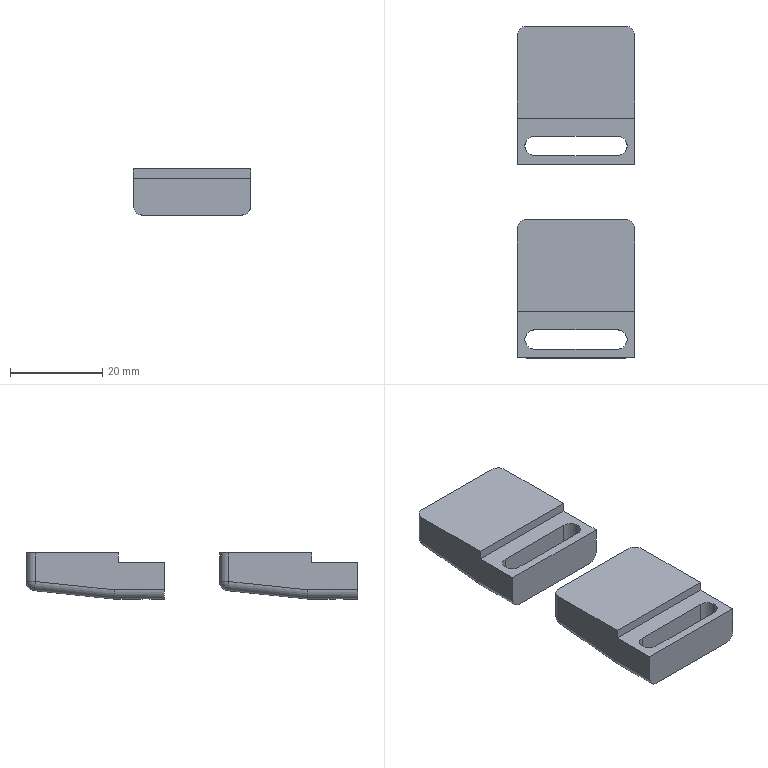NC program | NX | posted with a generic post | part box 25.5 x 72 x 10 mm
Whole program:
N10 G17 G21 G94 G90
(HOLE_MILLING , TOOL : D6)
N12 T12 M6
N14 G54
N16 G17 G0 G90 X0. Y-11. B0. C0. S9500 M3
N18 G43 Z30. H12
N20 Z0.5
N22 G94 G3 X1. Y-12. R1. F1250.
N24 X2. Y-11. R1.
N26 X2. Y-11. Z-0.5 I-2. J0.
N28 X2. Y-11. Z-1.5 I-2. J0.
N30 X2. Y-11. Z-2.5 I-2. J0.
N32 X2. Y-11. Z-3.5 I-2. J0.
N34 X2. Y-11. Z-4.5 I-2. J0.
N36 X2. Y-11. Z-5.5 I-2. J0.
N38 X2. Y-11. Z-6.5 I-2. J0.
N40 X2. Y-11. Z-7.5 I-2. J0.
N42 X2. Y-11. Z-8.5 I-2. J0.
N44 X2. Y-11. Z-9.5 I-2. J0.
N46 X2. Y-11. Z-10.5 I-2. J0.
N48 X2. Y-11. Z-11.5 I-2. J0.
N50 X2. Y-11. Z-12.5 I-2. J0.
N52 X2. Y-11. Z-13.5 I-2. J0.
N54 X2. Y-11. Z-14.5 I-2. J0.
N56 X2. Y-11. Z-15.5 I-2. J0.
N58 X2. Y-11. Z-16.5 I-2. J0.
N60 X2. Y-11. Z-17.5 I-2. J0.
N62 X2. Y-11. Z-18.5 I-2. J0.
N64 X2. Y-11. Z-19.5 I-2. J0.
N66 X-2. Y-11. Z-20. I-2. J0.
N68 X0. Y-13. R2.
N70 X-2. Y-11. R-2.
N72 X-1. Y-12. R1.
N74 X0. Y-11. R1.
N76 G0 Z30.
N78 M5
N80 M2